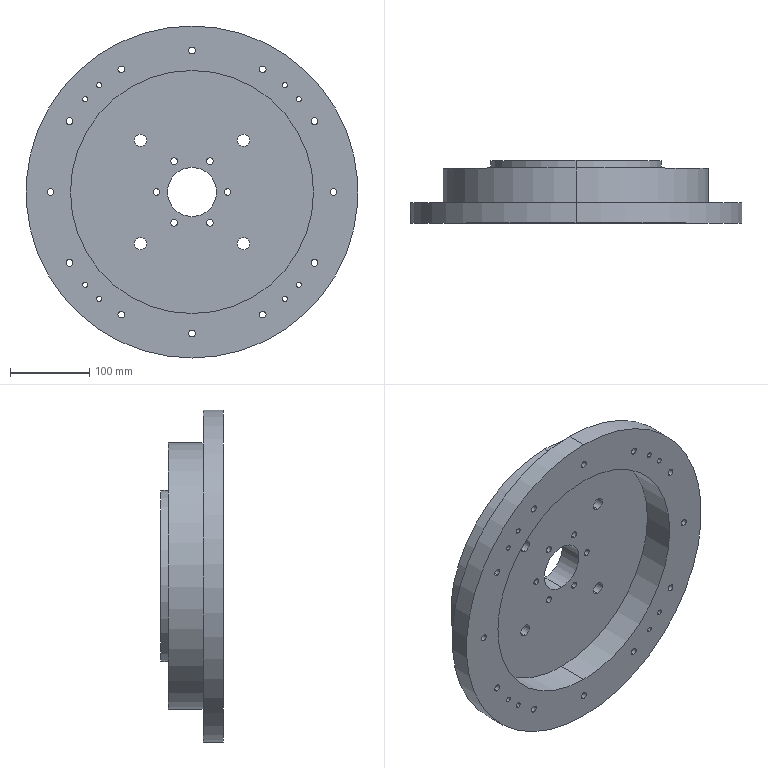Part | STEP file | 1 solid | 78 faces | box 419 x 78.97 x 419 mm | volume 4583187 mm3 | cylinder 72 | plane 6 | commonest cylinder face diameters 8.5 x36 6.5 x16 15.5 x8 62 x2 108 x2 215.9 x2